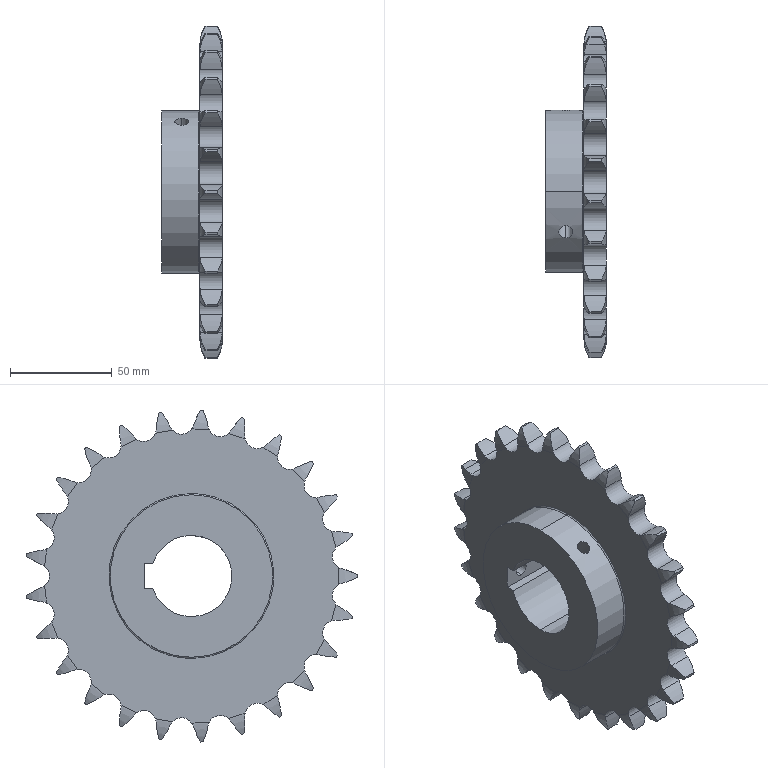Part | SolidWorks | features ICE 3, BaseBody 1, CirPattern 1, HoleWzd 1 | 1 solid | 177 faces | box 30.001 x 163.166 x 163.486 mm | volume 245205 mm3 | cylinder 119 | spline 52 | plane 6 | commonest cylinder face diameters 78.214 x51 12.191 x34 163.737 x25 6.8 x4 40 x3 80 x2